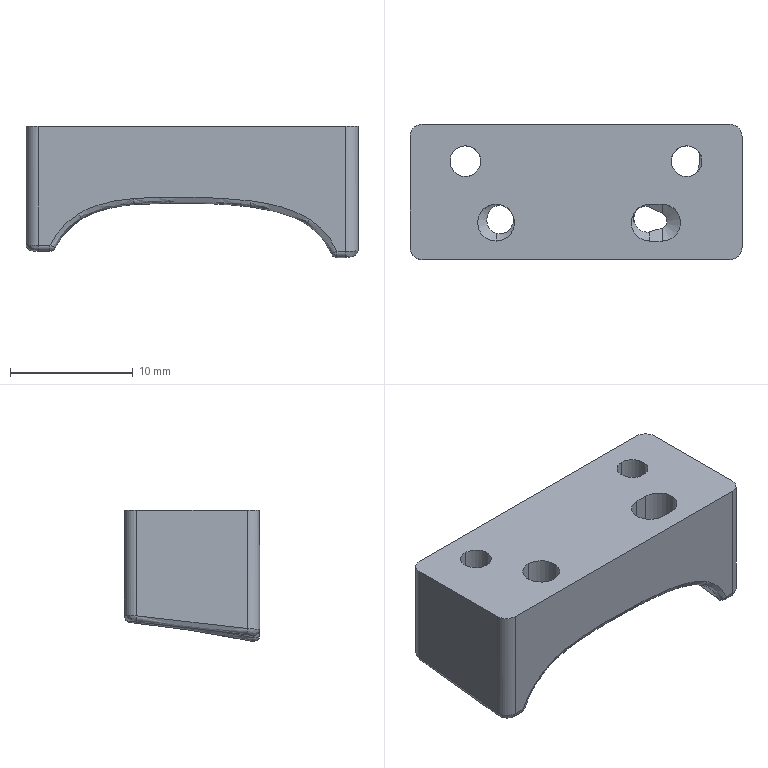Part | 1 solid | 62 faces | box 27 x 11 x 10.668 mm | volume 1858 mm3 | spline 26 | cylinder 16 | plane 9 | cone 7 | sphere 4 | commonest cylinder face diameters 1 x4 2 x4 2.5 x4 3 x4